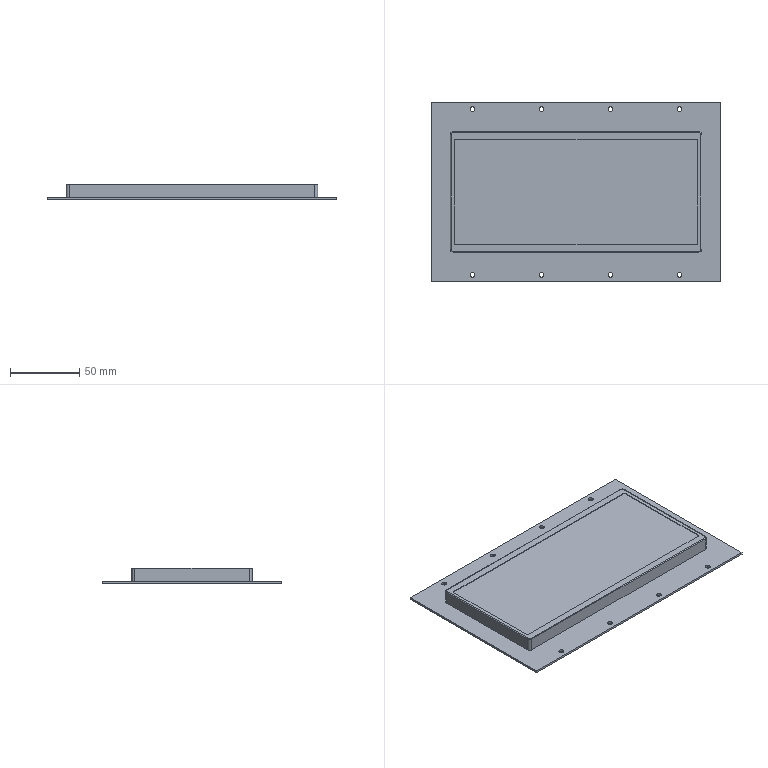Part | STEP file | 6151211W | 1 solid | 40 faces | box 210 x 130 x 11.5 mm | volume 192424 mm3 | cylinder 20 | plane 16 | torus 4 | commonest cylinder face diameters 3.5 x8 1 x4 2 x4 4 x4
STEP:
#1=CARTESIAN_POINT('',(-73.25,-60.,1.5));
#2=VERTEX_POINT('',#1);
#3=CARTESIAN_POINT('',(-75.,-60.,1.5));
#4=DIRECTION('',(0.,0.,1.));
#5=DIRECTION('',(1.,0.,0.));
#6=AXIS2_PLACEMENT_3D('',#3,#4,#5);
#7=CIRCLE('',#6,1.75);
#8=EDGE_CURVE('',#2,#2,#7,.T.);
#9=ORIENTED_EDGE('',*,*,#8,.F.);
#10=EDGE_LOOP('',(#9));
#11=FACE_BOUND('',#10,.T.);
#12=CARTESIAN_POINT('',(76.75,-60.,1.5));
#13=VERTEX_POINT('',#12);
#14=CARTESIAN_POINT('',(75.,-60.,1.5));
#15=DIRECTION('',(0.,0.,1.));
#16=DIRECTION('',(1.,0.,0.));
#17=AXIS2_PLACEMENT_3D('',#14,#15,#16);
#18=CIRCLE('',#17,1.75);
#19=EDGE_CURVE('',#13,#13,#18,.T.);
#20=ORIENTED_EDGE('',*,*,#19,.F.);
#21=EDGE_LOOP('',(#20));
#22=FACE_BOUND('',#21,.T.);
#23=CARTESIAN_POINT('',(26.75,60.,1.5));
#24=VERTEX_POINT('',#23);
#25=CARTESIAN_POINT('',(25.,60.,1.5));
#26=DIRECTION('',(0.,0.,1.));
#27=DIRECTION('',(1.,0.,0.));
#28=AXIS2_PLACEMENT_3D('',#25,#26,#27);
#29=CIRCLE('',#28,1.75);
#30=EDGE_CURVE('',#24,#24,#29,.T.);
#31=ORIENTED_EDGE('',*,*,#30,.F.);
#32=EDGE_LOOP('',(#31));
#33=FACE_BOUND('',#32,.T.);
#34=CARTESIAN_POINT('',(-23.25,60.,1.5));
#35=VERTEX_POINT('',#34);
#36=CARTESIAN_POINT('',(-25.,60.,1.5));
#37=DIRECTION('',(0.,0.,1.));
#38=DIRECTION('',(1.,0.,0.));
#39=AXIS2_PLACEMENT_3D('',#36,#37,#38);
#40=CIRCLE('',#39,1.75);
#41=EDGE_CURVE('',#35,#35,#40,.T.);
#42=ORIENTED_EDGE('',*,*,#41,.F.);
#43=EDGE_LOOP('',(#42));
#44=FACE_BOUND('',#43,.T.);
#45=CARTESIAN_POINT('',(-23.25,-60.,1.5));
#46=VERTEX_POINT('',#45);
#47=CARTESIAN_POINT('',(-25.,-60.,1.5));
#48=DIRECTION('',(0.,0.,1.));
#49=DIRECTION('',(1.,0.,0.));
#50=AXIS2_PLACEMENT_3D('',#47,#48,#49);
#51=CIRCLE('',#50,1.75);
#52=EDGE_CURVE('',#46,#46,#51,.T.);
#53=ORIENTED_EDGE('',*,*,#52,.F.);
#54=EDGE_LOOP('',(#53));
#55=FACE_BOUND('',#54,.T.);
#56=CARTESIAN_POINT('',(26.75,-60.,1.5));
#57=VERTEX_POINT('',#56);
#58=CARTESIAN_POINT('',(25.,-60.,1.5));
#59=DIRECTION('',(0.,0.,1.));
#60=DIRECTION('',(1.,0.,0.));
#61=AXIS2_PLACEMENT_3D('',#58,#59,#60);
#62=CIRCLE('',#61,1.75);
#63=EDGE_CURVE('',#57,#57,#62,.T.);
#64=ORIENTED_EDGE('',*,*,#63,.F.);
#65=EDGE_LOOP('',(#64));
#66=FACE_BOUND('',#65,.T.);
#67=CARTESIAN_POINT('',(76.75,60.,1.5));
#68=VERTEX_POINT('',#67);
#69=CARTESIAN_POINT('',(75.,60.,1.5));
#70=DIRECTION('',(0.,0.,1.));
#71=DIRECTION('',(1.,0.,0.));
#72=AXIS2_PLACEMENT_3D('',#69,#70,#71);
#73=CIRCLE('',#72,1.75);
#74=EDGE_CURVE('',#68,#68,#73,.T.);
#75=ORIENTED_EDGE('',*,*,#74,.F.);
#76=EDGE_LOOP('',(#75));
#77=FACE_BOUND('',#76,.T.);
#78=CARTESIAN_POINT('',(-73.25,60.,1.5));
#79=VERTEX_POINT('',#78);
#80=CARTESIAN_POINT('',(-75.,60.,1.5));
#81=DIRECTION('',(0.,0.,1.));
#82=DIRECTION('',(1.,0.,0.));
#83=AXIS2_PLACEMENT_3D('',#80,#81,#82);
#84=CIRCLE('',#83,1.75);
#85=EDGE_CURVE('',#79,#79,#84,.T.);
#86=ORIENTED_EDGE('',*,*,#85,.F.);
#87=EDGE_LOOP('',(#86));
#88=FACE_BOUND('',#87,.T.);
#89=CARTESIAN_POINT('',(-105.,65.,1.5));
#90=VERTEX_POINT('',#89);
#91=CARTESIAN_POINT('',(-105.,-65.,1.5));
#92=VERTEX_POINT('',#91);
#93=CARTESIAN_POINT('',(-105.,65.,1.5));
#94=DIRECTION('',(0.,-1.,0.));
#95=VECTOR('',#94,1000.);
#96=LINE('',#93,#95);
#97=EDGE_CURVE('',#90,#92,#96,.T.);
#98=ORIENTED_EDGE('',*,*,#97,.T.);
#99=CARTESIAN_POINT('',(105.,-65.,1.5));
#100=VERTEX_POINT('',#99);
#101=CARTESIAN_POINT('',(-105.,-65.,1.5));
#102=DIRECTION('',(1.,0.,0.));
#103=VECTOR('',#102,1000.);
#104=LINE('',#101,#103);
#105=EDGE_CURVE('',#92,#100,#104,.T.);
#106=ORIENTED_EDGE('',*,*,#105,.T.);
#107=CARTESIAN_POINT('',(105.,65.,1.5));
#108=VERTEX_POINT('',#107);
#109=CARTESIAN_POINT('',(105.,65.,1.5));
#110=DIRECTION('',(0.,1.,0.));
#111=VECTOR('',#110,1000.);
#112=LINE('',#109,#111);
#113=EDGE_CURVE('',#100,#108,#112,.T.);
#114=ORIENTED_EDGE('',*,*,#113,.T.);
#115=CARTESIAN_POINT('',(-105.,65.,1.5));
#116=DIRECTION('',(-1.,0.,0.));
#117=VECTOR('',#116,1000.);
#118=LINE('',#115,#117);
#119=EDGE_CURVE('',#108,#90,#118,.T.);
#120=ORIENTED_EDGE('',*,*,#119,.T.);
#121=EDGE_LOOP('',(#98,#106,#114,#120));
#122=FACE_OUTER_BOUND('',#121,.T.);
#123=CARTESIAN_POINT('',(89.,43.5,1.5));
#124=VERTEX_POINT('',#123);
#125=CARTESIAN_POINT('',(-89.,43.5,1.5));
#126=VERTEX_POINT('',#125);
#127=CARTESIAN_POINT('',(-89.,43.5,1.5));
#128=DIRECTION('',(-1.,0.,0.));
#129=VECTOR('',#128,1000.);
#130=LINE('',#127,#129);
#131=EDGE_CURVE('',#124,#126,#130,.T.);
#132=ORIENTED_EDGE('',*,*,#131,.F.);
#133=CARTESIAN_POINT('',(91.,41.5,1.5));
#134=VERTEX_POINT('',#133);
#135=CARTESIAN_POINT('',(89.,41.5,1.5));
#136=DIRECTION('',(0.,0.,1.));
#137=DIRECTION('',(1.,0.,0.));
#138=AXIS2_PLACEMENT_3D('',#135,#136,#137);
#139=CIRCLE('',#138,2.);
#140=EDGE_CURVE('',#134,#124,#139,.T.);
#141=ORIENTED_EDGE('',*,*,#140,.F.);
#142=CARTESIAN_POINT('',(91.,-41.5,1.5));
#143=VERTEX_POINT('',#142);
#144=CARTESIAN_POINT('',(91.,41.5,1.5));
#145=DIRECTION('',(0.,1.,0.));
#146=VECTOR('',#145,1000.);
#147=LINE('',#144,#146);
#148=EDGE_CURVE('',#143,#134,#147,.T.);
#149=ORIENTED_EDGE('',*,*,#148,.F.);
#150=CARTESIAN_POINT('',(89.,-43.5,1.5));
#151=VERTEX_POINT('',#150);
#152=CARTESIAN_POINT('',(89.,-41.5,1.5));
#153=DIRECTION('',(0.,0.,1.));
#154=DIRECTION('',(1.,0.,0.));
#155=AXIS2_PLACEMENT_3D('',#152,#153,#154);
#156=CIRCLE('',#155,2.);
#157=EDGE_CURVE('',#151,#143,#156,.T.);
#158=ORIENTED_EDGE('',*,*,#157,.F.);
#159=CARTESIAN_POINT('',(-89.,-43.5,1.5));
#160=VERTEX_POINT('',#159);
#161=CARTESIAN_POINT('',(-89.,-43.5,1.5));
#162=DIRECTION('',(1.,0.,0.));
#163=VECTOR('',#162,1000.);
#164=LINE('',#161,#163);
#165=EDGE_CURVE('',#160,#151,#164,.T.);
#166=ORIENTED_EDGE('',*,*,#165,.F.);
#167=CARTESIAN_POINT('',(-91.,-41.5,1.5));
#168=VERTEX_POINT('',#167);
#169=CARTESIAN_POINT('',(-89.,-41.5,1.5));
#170=DIRECTION('',(0.,0.,1.));
#171=DIRECTION('',(1.,0.,0.));
#172=AXIS2_PLACEMENT_3D('',#169,#170,#171);
#173=CIRCLE('',#172,2.);
#174=EDGE_CURVE('',#168,#160,#173,.T.);
#175=ORIENTED_EDGE('',*,*,#174,.F.);
#176=CARTESIAN_POINT('',(-91.,41.5,1.5));
#177=VERTEX_POINT('',#176);
#178=CARTESIAN_POINT('',(-91.,41.5,1.5));
#179=DIRECTION('',(0.,-1.,0.));
#180=VECTOR('',#179,1000.);
#181=LINE('',#178,#180);
#182=EDGE_CURVE('',#177,#168,#181,.T.);
#183=ORIENTED_EDGE('',*,*,#182,.F.);
#184=CARTESIAN_POINT('',(-89.,41.5,1.5));
#185=DIRECTION('',(0.,0.,1.));
#186=DIRECTION('',(1.,0.,0.));
#187=AXIS2_PLACEMENT_3D('',#184,#185,#186);
#188=CIRCLE('',#187,2.);
#189=EDGE_CURVE('',#126,#177,#188,.T.);
#190=ORIENTED_EDGE('',*,*,#189,.F.);
#191=EDGE_LOOP('',(#132,#141,#149,#158,#166,#175,#183,#190));
#192=FACE_BOUND('',#191,.T.);
#193=CARTESIAN_POINT('',(-105.,-65.,1.5));
#194=DIRECTION('',(0.,0.,1.));
#195=DIRECTION('',(1.,0.,0.));
#196=AXIS2_PLACEMENT_3D('',#193,#194,#195);
#197=PLANE('',#196);
#198=ADVANCED_FACE('',(#11,#22,#33,#44,#55,#66,#77,#88,#122,#192),#197,.T.);
#199=CARTESIAN_POINT('',(-105.,65.,0.));
#200=VERTEX_POINT('',#199);
#201=CARTESIAN_POINT('',(-105.,-65.,0.));
#202=VERTEX_POINT('',#201);
#203=CARTESIAN_POINT('',(-105.,65.,0.));
#204=DIRECTION('',(0.,-1.,0.));
#205=VECTOR('',#204,1000.);
#206=LINE('',#203,#205);
#207=EDGE_CURVE('',#200,#202,#206,.T.);
#208=ORIENTED_EDGE('',*,*,#207,.T.);
#209=CARTESIAN_POINT('',(-105.,-65.,1.5));
#210=DIRECTION('',(0.,0.,-1.));
#211=VECTOR('',#210,1000.);
#212=LINE('',#209,#211);
#213=EDGE_CURVE('',#92,#202,#212,.T.);
#214=ORIENTED_EDGE('',*,*,#213,.F.);
#215=ORIENTED_EDGE('',*,*,#97,.F.);
#216=CARTESIAN_POINT('',(-105.,65.,1.5));
#217=DIRECTION('',(0.,0.,-1.));
#218=VECTOR('',#217,1000.);
#219=LINE('',#216,#218);
#220=EDGE_CURVE('',#90,#200,#219,.T.);
#221=ORIENTED_EDGE('',*,*,#220,.T.);
#222=EDGE_LOOP('',(#208,#214,#215,#221));
#223=FACE_OUTER_BOUND('',#222,.T.);
#224=CARTESIAN_POINT('',(-105.,65.,1.5));
#225=DIRECTION('',(1.,0.,0.));
#226=DIRECTION('',(0.,1.,0.));
#227=AXIS2_PLACEMENT_3D('',#224,#225,#226);
#228=PLANE('',#227);
#229=ADVANCED_FACE('',(#223),#228,.F.);
#230=CARTESIAN_POINT('',(105.,-65.,0.));
#231=VERTEX_POINT('',#230);
#232=CARTESIAN_POINT('',(-105.,-65.,0.));
#233=DIRECTION('',(1.,0.,0.));
#234=VECTOR('',#233,1000.);
#235=LINE('',#232,#234);
#236=EDGE_CURVE('',#202,#231,#235,.T.);
#237=ORIENTED_EDGE('',*,*,#236,.T.);
#238=CARTESIAN_POINT('',(105.,-65.,1.5));
#239=DIRECTION('',(0.,0.,-1.));
#240=VECTOR('',#239,1000.);
#241=LINE('',#238,#240);
#242=EDGE_CURVE('',#100,#231,#241,.T.);
#243=ORIENTED_EDGE('',*,*,#242,.F.);
#244=ORIENTED_EDGE('',*,*,#105,.F.);
#245=ORIENTED_EDGE('',*,*,#213,.T.);
#246=EDGE_LOOP('',(#237,#243,#244,#245));
#247=FACE_OUTER_BOUND('',#246,.T.);
#248=CARTESIAN_POINT('',(-105.,-65.,1.5));
#249=DIRECTION('',(0.,1.,0.));
#250=DIRECTION('',(0.,0.,1.));
#251=AXIS2_PLACEMENT_3D('',#248,#249,#250);
#252=PLANE('',#251);
#253=ADVANCED_FACE('',(#247),#252,.F.);
#254=CARTESIAN_POINT('',(105.,65.,0.));
#255=VERTEX_POINT('',#254);
#256=CARTESIAN_POINT('',(105.,65.,0.));
#257=DIRECTION('',(0.,1.,0.));
#258=VECTOR('',#257,1000.);
#259=LINE('',#256,#258);
#260=EDGE_CURVE('',#231,#255,#259,.T.);
#261=ORIENTED_EDGE('',*,*,#260,.T.);
#262=CARTESIAN_POINT('',(105.,65.,1.5));
#263=DIRECTION('',(0.,0.,-1.));
#264=VECTOR('',#263,1000.);
#265=LINE('',#262,#264);
#266=EDGE_CURVE('',#108,#255,#265,.T.);
#267=ORIENTED_EDGE('',*,*,#266,.F.);
#268=ORIENTED_EDGE('',*,*,#113,.F.);
#269=ORIENTED_EDGE('',*,*,#242,.T.);
#270=EDGE_LOOP('',(#261,#267,#268,#269));
#271=FACE_OUTER_BOUND('',#270,.T.);
#272=CARTESIAN_POINT('',(105.,65.,1.5));
#273=DIRECTION('',(-1.,0.,0.));
#274=DIRECTION('',(0.,-1.,0.));
#275=AXIS2_PLACEMENT_3D('',#272,#273,#274);
#276=PLANE('',#275);
#277=ADVANCED_FACE('',(#271),#276,.F.);
#278=CARTESIAN_POINT('',(-105.,65.,0.));
#279=DIRECTION('',(-1.,0.,0.));
#280=VECTOR('',#279,1000.);
#281=LINE('',#278,#280);
#282=EDGE_CURVE('',#255,#200,#281,.T.);
#283=ORIENTED_EDGE('',*,*,#282,.T.);
#284=ORIENTED_EDGE('',*,*,#220,.F.);
#285=ORIENTED_EDGE('',*,*,#119,.F.);
#286=ORIENTED_EDGE('',*,*,#266,.T.);
#287=EDGE_LOOP('',(#283,#284,#285,#286));
#288=FACE_OUTER_BOUND('',#287,.T.);
#289=CARTESIAN_POINT('',(-105.,65.,1.5));
#290=DIRECTION('',(0.,-1.,0.));
#291=DIRECTION('',(0.,0.,-1.));
#292=AXIS2_PLACEMENT_3D('',#289,#290,#291);
#293=PLANE('',#292);
#294=ADVANCED_FACE('',(#288),#293,.F.);
#295=CARTESIAN_POINT('',(-73.25,-60.,0.));
#296=VERTEX_POINT('',#295);
#297=CARTESIAN_POINT('',(-75.,-60.,0.));
#298=DIRECTION('',(0.,0.,-1.));
#299=DIRECTION('',(1.,0.,0.));
#300=AXIS2_PLACEMENT_3D('',#297,#298,#299);
#301=CIRCLE('',#300,1.75);
#302=EDGE_CURVE('',#296,#296,#301,.T.);
#303=ORIENTED_EDGE('',*,*,#302,.F.);
#304=EDGE_LOOP('',(#303));
#305=FACE_BOUND('',#304,.T.);
#306=CARTESIAN_POINT('',(76.75,-60.,0.));
#307=VERTEX_POINT('',#306);
#308=CARTESIAN_POINT('',(75.,-60.,0.));
#309=DIRECTION('',(0.,0.,-1.));
#310=DIRECTION('',(1.,0.,0.));
#311=AXIS2_PLACEMENT_3D('',#308,#309,#310);
#312=CIRCLE('',#311,1.75);
#313=EDGE_CURVE('',#307,#307,#312,.T.);
#314=ORIENTED_EDGE('',*,*,#313,.F.);
#315=EDGE_LOOP('',(#314));
#316=FACE_BOUND('',#315,.T.);
#317=CARTESIAN_POINT('',(23.25,60.,0.));
#318=VERTEX_POINT('',#317);
#319=CARTESIAN_POINT('',(25.,60.,0.));
#320=DIRECTION('',(0.,0.,-1.));
#321=DIRECTION('',(-1.,0.,0.));
#322=AXIS2_PLACEMENT_3D('',#319,#320,#321);
#323=CIRCLE('',#322,1.75);
#324=EDGE_CURVE('',#318,#318,#323,.T.);
#325=ORIENTED_EDGE('',*,*,#324,.F.);
#326=EDGE_LOOP('',(#325));
#327=FACE_BOUND('',#326,.T.);
#328=CARTESIAN_POINT('',(-26.75,60.,0.));
#329=VERTEX_POINT('',#328);
#330=CARTESIAN_POINT('',(-25.,60.,0.));
#331=DIRECTION('',(0.,0.,-1.));
#332=DIRECTION('',(-1.,0.,0.));
#333=AXIS2_PLACEMENT_3D('',#330,#331,#332);
#334=CIRCLE('',#333,1.75);
#335=EDGE_CURVE('',#329,#329,#334,.T.);
#336=ORIENTED_EDGE('',*,*,#335,.F.);
#337=EDGE_LOOP('',(#336));
#338=FACE_BOUND('',#337,.T.);
#339=CARTESIAN_POINT('',(-23.25,-60.,0.));
#340=VERTEX_POINT('',#339);
#341=CARTESIAN_POINT('',(-25.,-60.,0.));
#342=DIRECTION('',(0.,0.,-1.));
#343=DIRECTION('',(1.,0.,0.));
#344=AXIS2_PLACEMENT_3D('',#341,#342,#343);
#345=CIRCLE('',#344,1.75);
#346=EDGE_CURVE('',#340,#340,#345,.T.);
#347=ORIENTED_EDGE('',*,*,#346,.F.);
#348=EDGE_LOOP('',(#347));
#349=FACE_BOUND('',#348,.T.);
#350=CARTESIAN_POINT('',(26.75,-60.,0.));
#351=VERTEX_POINT('',#350);
#352=CARTESIAN_POINT('',(25.,-60.,0.));
#353=DIRECTION('',(0.,0.,-1.));
#354=DIRECTION('',(1.,0.,0.));
#355=AXIS2_PLACEMENT_3D('',#352,#353,#354);
#356=CIRCLE('',#355,1.75);
#357=EDGE_CURVE('',#351,#351,#356,.T.);
#358=ORIENTED_EDGE('',*,*,#357,.F.);
#359=EDGE_LOOP('',(#358));
#360=FACE_BOUND('',#359,.T.);
#361=CARTESIAN_POINT('',(73.25,60.,0.));
#362=VERTEX_POINT('',#361);
#363=CARTESIAN_POINT('',(75.,60.,0.));
#364=DIRECTION('',(0.,0.,-1.));
#365=DIRECTION('',(-1.,0.,0.));
#366=AXIS2_PLACEMENT_3D('',#363,#364,#365);
#367=CIRCLE('',#366,1.75);
#368=EDGE_CURVE('',#362,#362,#367,.T.);
#369=ORIENTED_EDGE('',*,*,#368,.F.);
#370=EDGE_LOOP('',(#369));
#371=FACE_BOUND('',#370,.T.);
#372=CARTESIAN_POINT('',(-76.75,60.,0.));
#373=VERTEX_POINT('',#372);
#374=CARTESIAN_POINT('',(-75.,60.,0.));
#375=DIRECTION('',(0.,0.,-1.));
#376=DIRECTION('',(-1.,0.,0.));
#377=AXIS2_PLACEMENT_3D('',#374,#375,#376);
#378=CIRCLE('',#377,1.75);
#379=EDGE_CURVE('',#373,#373,#378,.T.);
#380=ORIENTED_EDGE('',*,*,#379,.F.);
#381=EDGE_LOOP('',(#380));
#382=FACE_BOUND('',#381,.T.);
#383=ORIENTED_EDGE('',*,*,#207,.F.);
#384=ORIENTED_EDGE('',*,*,#282,.F.);
#385=ORIENTED_EDGE('',*,*,#260,.F.);
#386=ORIENTED_EDGE('',*,*,#236,.F.);
#387=EDGE_LOOP('',(#383,#384,#385,#386));
#388=FACE_OUTER_BOUND('',#387,.T.);
#389=CARTESIAN_POINT('',(-105.,-65.,0.));
#390=DIRECTION('',(0.,0.,1.));
#391=DIRECTION('',(1.,0.,0.));
#392=AXIS2_PLACEMENT_3D('',#389,#390,#391);
#393=PLANE('',#392);
#394=ADVANCED_FACE('',(#305,#316,#327,#338,#349,#360,#371,#382,#388),#393,.F.);
#395=CARTESIAN_POINT('',(89.,43.5,11.));
#396=VERTEX_POINT('',#395);
#397=CARTESIAN_POINT('',(89.,43.5,11.5));
#398=DIRECTION('',(0.,0.,-1.));
#399=VECTOR('',#398,1000.);
#400=LINE('',#397,#399);
#401=EDGE_CURVE('',#396,#124,#400,.T.);
#402=ORIENTED_EDGE('',*,*,#401,.F.);
#403=CARTESIAN_POINT('',(91.,41.5,11.));
#404=VERTEX_POINT('',#403);
#405=CARTESIAN_POINT('',(89.,41.5,11.));
#406=DIRECTION('',(0.,0.,-1.));
#407=DIRECTION('',(1.,0.,0.));
#408=AXIS2_PLACEMENT_3D('',#405,#406,#407);
#409=CIRCLE('',#408,2.);
#410=EDGE_CURVE('',#396,#404,#409,.T.);
#411=ORIENTED_EDGE('',*,*,#410,.T.);
#412=CARTESIAN_POINT('',(91.,41.5,11.5));
#413=DIRECTION('',(0.,0.,-1.));
#414=VECTOR('',#413,1000.);
#415=LINE('',#412,#414);
#416=EDGE_CURVE('',#404,#134,#415,.T.);
#417=ORIENTED_EDGE('',*,*,#416,.T.);
#418=ORIENTED_EDGE('',*,*,#140,.T.);
#419=EDGE_LOOP('',(#402,#411,#417,#418));
#420=FACE_OUTER_BOUND('',#419,.T.);
#421=CARTESIAN_POINT('',(89.,41.5,11.5));
#422=DIRECTION('',(0.,0.,-1.));
#423=DIRECTION('',(-1.,0.,0.));
#424=AXIS2_PLACEMENT_3D('',#421,#422,#423);
#425=CYLINDRICAL_SURFACE('',#424,2.);
#426=ADVANCED_FACE('',(#420),#425,.T.);
#427=CARTESIAN_POINT('',(-89.,43.5,11.));
#428=VERTEX_POINT('',#427);
#429=CARTESIAN_POINT('',(-89.,43.5,11.5));
#430=DIRECTION('',(0.,0.,-1.));
#431=VECTOR('',#430,1000.);
#432=LINE('',#429,#431);
#433=EDGE_CURVE('',#428,#126,#432,.T.);
#434=ORIENTED_EDGE('',*,*,#433,.F.);
#435=CARTESIAN_POINT('',(89.,43.5,11.));
#436=DIRECTION('',(1.,0.,0.));
#437=VECTOR('',#436,1000.);
#438=LINE('',#435,#437);
#439=EDGE_CURVE('',#428,#396,#438,.T.);
#440=ORIENTED_EDGE('',*,*,#439,.T.);
#441=ORIENTED_EDGE('',*,*,#401,.T.);
#442=ORIENTED_EDGE('',*,*,#131,.T.);
#443=EDGE_LOOP('',(#434,#440,#441,#442));
#444=FACE_OUTER_BOUND('',#443,.T.);
#445=CARTESIAN_POINT('',(-89.,43.5,11.5));
#446=DIRECTION('',(0.,-1.,0.));
#447=DIRECTION('',(1.,0.,0.));
#448=AXIS2_PLACEMENT_3D('',#445,#446,#447);
#449=PLANE('',#448);
#450=ADVANCED_FACE('',(#444),#449,.F.);
#451=CARTESIAN_POINT('',(-91.,41.5,11.));
#452=VERTEX_POINT('',#451);
#453=CARTESIAN_POINT('',(-91.,41.5,11.5));
#454=DIRECTION('',(0.,0.,-1.));
#455=VECTOR('',#454,1000.);
#456=LINE('',#453,#455);
#457=EDGE_CURVE('',#452,#177,#456,.T.);
#458=ORIENTED_EDGE('',*,*,#457,.F.);
#459=CARTESIAN_POINT('',(-89.,41.5,11.));
#460=DIRECTION('',(0.,0.,-1.));
#461=DIRECTION('',(1.,0.,0.));
#462=AXIS2_PLACEMENT_3D('',#459,#460,#461);
#463=CIRCLE('',#462,2.);
#464=EDGE_CURVE('',#452,#428,#463,.T.);
#465=ORIENTED_EDGE('',*,*,#464,.T.);
#466=ORIENTED_EDGE('',*,*,#433,.T.);
#467=ORIENTED_EDGE('',*,*,#189,.T.);
#468=EDGE_LOOP('',(#458,#465,#466,#467));
#469=FACE_OUTER_BOUND('',#468,.T.);
#470=CARTESIAN_POINT('',(-89.,41.5,11.5));
#471=DIRECTION('',(0.,0.,-1.));
#472=DIRECTION('',(-1.,0.,0.));
#473=AXIS2_PLACEMENT_3D('',#470,#471,#472);
#474=CYLINDRICAL_SURFACE('',#473,2.);
#475=ADVANCED_FACE('',(#469),#474,.T.);
#476=CARTESIAN_POINT('',(-91.,-41.5,11.));
#477=VERTEX_POINT('',#476);
#478=CARTESIAN_POINT('',(-91.,-41.5,11.5));
#479=DIRECTION('',(0.,0.,-1.));
#480=VECTOR('',#479,1000.);
#481=LINE('',#478,#480);
#482=EDGE_CURVE('',#477,#168,#481,.T.);
#483=ORIENTED_EDGE('',*,*,#482,.F.);
#484=CARTESIAN_POINT('',(-91.,41.5,11.));
#485=DIRECTION('',(0.,1.,0.));
#486=VECTOR('',#485,1000.);
#487=LINE('',#484,#486);
#488=EDGE_CURVE('',#477,#452,#487,.T.);
#489=ORIENTED_EDGE('',*,*,#488,.T.);
#490=ORIENTED_EDGE('',*,*,#457,.T.);
#491=ORIENTED_EDGE('',*,*,#182,.T.);
#492=EDGE_LOOP('',(#483,#489,#490,#491));
#493=FACE_OUTER_BOUND('',#492,.T.);
#494=CARTESIAN_POINT('',(-91.,41.5,11.5));
#495=DIRECTION('',(1.,0.,0.));
#496=DIRECTION('',(0.,1.,0.));
#497=AXIS2_PLACEMENT_3D('',#494,#495,#496);
#498=PLANE('',#497);
#499=ADVANCED_FACE('',(#493),#498,.F.);
#500=CARTESIAN_POINT('',(-89.,-43.5,11.));
#501=VERTEX_POINT('',#500);
#502=CARTESIAN_POINT('',(-89.,-43.5,11.5));
#503=DIRECTION('',(0.,0.,-1.));
#504=VECTOR('',#503,1000.);
#505=LINE('',#502,#504);
#506=EDGE_CURVE('',#501,#160,#505,.T.);
#507=ORIENTED_EDGE('',*,*,#506,.F.);
#508=CARTESIAN_POINT('',(-89.,-41.5,11.));
#509=DIRECTION('',(0.,0.,-1.));
#510=DIRECTION('',(1.,0.,0.));
#511=AXIS2_PLACEMENT_3D('',#508,#509,#510);
#512=CIRCLE('',#511,2.);
#513=EDGE_CURVE('',#501,#477,#512,.T.);
#514=ORIENTED_EDGE('',*,*,#513,.T.);
#515=ORIENTED_EDGE('',*,*,#482,.T.);
#516=ORIENTED_EDGE('',*,*,#174,.T.);
#517=EDGE_LOOP('',(#507,#514,#515,#516));
#518=FACE_OUTER_BOUND('',#517,.T.);
#519=CARTESIAN_POINT('',(-89.,-41.5,11.5));
#520=DIRECTION('',(0.,0.,-1.));
#521=DIRECTION('',(-1.,0.,0.));
#522=AXIS2_PLACEMENT_3D('',#519,#520,#521);
#523=CYLINDRICAL_SURFACE('',#522,2.);
#524=ADVANCED_FACE('',(#518),#523,.T.);
#525=CARTESIAN_POINT('',(89.,-43.5,11.));
#526=VERTEX_POINT('',#525);
#527=CARTESIAN_POINT('',(89.,-43.5,11.5));
#528=DIRECTION('',(0.,0.,-1.));
#529=VECTOR('',#528,1000.);
#530=LINE('',#527,#529);
#531=EDGE_CURVE('',#526,#151,#530,.T.);
#532=ORIENTED_EDGE('',*,*,#531,.F.);
#533=CARTESIAN_POINT('',(-89.,-43.5,11.));
#534=DIRECTION('',(-1.,0.,0.));
#535=VECTOR('',#534,1000.);
#536=LINE('',#533,#535);
#537=EDGE_CURVE('',#526,#501,#536,.T.);
#538=ORIENTED_EDGE('',*,*,#537,.T.);
#539=ORIENTED_EDGE('',*,*,#506,.T.);
#540=ORIENTED_EDGE('',*,*,#165,.T.);
#541=EDGE_LOOP('',(#532,#538,#539,#540));
#542=FACE_OUTER_BOUND('',#541,.T.);
#543=CARTESIAN_POINT('',(-89.,-43.5,11.5));
#544=DIRECTION('',(0.,1.,0.));
#545=DIRECTION('',(-1.,0.,0.));
#546=AXIS2_PLACEMENT_3D('',#543,#544,#545);
#547=PLANE('',#546);
#548=ADVANCED_FACE('',(#542),#547,.F.);
#549=CARTESIAN_POINT('',(91.,-41.5,11.));
#550=VERTEX_POINT('',#549);
#551=CARTESIAN_POINT('',(91.,-41.5,11.5));
#552=DIRECTION('',(0.,0.,-1.));
#553=VECTOR('',#552,1000.);
#554=LINE('',#551,#553);
#555=EDGE_CURVE('',#550,#143,#554,.T.);
#556=ORIENTED_EDGE('',*,*,#555,.F.);
#557=CARTESIAN_POINT('',(89.,-41.5,11.));
#558=DIRECTION('',(0.,0.,-1.));
#559=DIRECTION('',(1.,0.,0.));
#560=AXIS2_PLACEMENT_3D('',#557,#558,#559);
#561=CIRCLE('',#560,2.);
#562=EDGE_CURVE('',#550,#526,#561,.T.);
#563=ORIENTED_EDGE('',*,*,#562,.T.);
#564=ORIENTED_EDGE('',*,*,#531,.T.);
#565=ORIENTED_EDGE('',*,*,#157,.T.);
#566=EDGE_LOOP('',(#556,#563,#564,#565));
#567=FACE_OUTER_BOUND('',#566,.T.);
#568=CARTESIAN_POINT('',(89.,-41.5,11.5));
#569=DIRECTION('',(0.,0.,-1.));
#570=DIRECTION('',(-1.,0.,0.));
#571=AXIS2_PLACEMENT_3D('',#568,#569,#570);
#572=CYLINDRICAL_SURFACE('',#571,2.);
#573=ADVANCED_FACE('',(#567),#572,.T.);
#574=ORIENTED_EDGE('',*,*,#416,.F.);
#575=CARTESIAN_POINT('',(91.,-41.5,11.));
#576=DIRECTION('',(0.,-1.,0.));
#577=VECTOR('',#576,1000.);
#578=LINE('',#575,#577);
#579=EDGE_CURVE('',#404,#550,#578,.T.);
#580=ORIENTED_EDGE('',*,*,#579,.T.);
#581=ORIENTED_EDGE('',*,*,#555,.T.);
#582=ORIENTED_EDGE('',*,*,#148,.T.);
#583=EDGE_LOOP('',(#574,#580,#581,#582));
#584=FACE_OUTER_BOUND('',#583,.T.);
#585=CARTESIAN_POINT('',(91.,41.5,11.5));
#586=DIRECTION('',(-1.,0.,0.));
#587=DIRECTION('',(0.,-1.,0.));
#588=AXIS2_PLACEMENT_3D('',#585,#586,#587);
#589=PLANE('',#588);
#590=ADVANCED_FACE('',(#584),#589,.F.);
#591=CARTESIAN_POINT('',(89.,43.,11.5));
#592=VERTEX_POINT('',#591);
#593=CARTESIAN_POINT('',(-89.,43.,11.5));
#594=VERTEX_POINT('',#593);
#595=CARTESIAN_POINT('',(-89.,43.,11.5));
#596=DIRECTION('',(-1.,0.,0.));
#597=VECTOR('',#596,1000.);
#598=LINE('',#595,#597);
#599=EDGE_CURVE('',#592,#594,#598,.T.);
#600=ORIENTED_EDGE('',*,*,#599,.T.);
#601=CARTESIAN_POINT('',(-90.5,41.5,11.5));
#602=VERTEX_POINT('',#601);
#603=CARTESIAN_POINT('',(-89.,41.5,11.5));
#604=DIRECTION('',(0.,0.,1.));
#605=DIRECTION('',(1.,0.,0.));
#606=AXIS2_PLACEMENT_3D('',#603,#604,#605);
#607=CIRCLE('',#606,1.5);
#608=EDGE_CURVE('',#594,#602,#607,.T.);
#609=ORIENTED_EDGE('',*,*,#608,.T.);
#610=CARTESIAN_POINT('',(-90.5,-41.5,11.5));
#611=VERTEX_POINT('',#610);
#612=CARTESIAN_POINT('',(-90.5,-41.5,11.5));
#613=DIRECTION('',(0.,-1.,0.));
#614=VECTOR('',#613,1000.);
#615=LINE('',#612,#614);
#616=EDGE_CURVE('',#602,#611,#615,.T.);
#617=ORIENTED_EDGE('',*,*,#616,.T.);
#618=CARTESIAN_POINT('',(-89.,-43.,11.5));
#619=VERTEX_POINT('',#618);
#620=CARTESIAN_POINT('',(-89.,-41.5,11.5));
#621=DIRECTION('',(0.,0.,1.));
#622=DIRECTION('',(1.,0.,0.));
#623=AXIS2_PLACEMENT_3D('',#620,#621,#622);
#624=CIRCLE('',#623,1.5);
#625=EDGE_CURVE('',#611,#619,#624,.T.);
#626=ORIENTED_EDGE('',*,*,#625,.T.);
#627=CARTESIAN_POINT('',(89.,-43.,11.5));
#628=VERTEX_POINT('',#627);
#629=CARTESIAN_POINT('',(89.,-43.,11.5));
#630=DIRECTION('',(1.,0.,0.));
#631=VECTOR('',#630,1000.);
#632=LINE('',#629,#631);
#633=EDGE_CURVE('',#619,#628,#632,.T.);
#634=ORIENTED_EDGE('',*,*,#633,.T.);
#635=CARTESIAN_POINT('',(90.5,-41.5,11.5));
#636=VERTEX_POINT('',#635);
#637=CARTESIAN_POINT('',(89.,-41.5,11.5));
#638=DIRECTION('',(0.,0.,1.));
#639=DIRECTION('',(1.,0.,0.));
#640=AXIS2_PLACEMENT_3D('',#637,#638,#639);
#641=CIRCLE('',#640,1.5);
#642=EDGE_CURVE('',#628,#636,#641,.T.);
#643=ORIENTED_EDGE('',*,*,#642,.T.);
#644=CARTESIAN_POINT('',(90.5,41.5,11.5));
#645=VERTEX_POINT('',#644);
#646=CARTESIAN_POINT('',(90.5,41.5,11.5));
#647=DIRECTION('',(0.,1.,0.));
#648=VECTOR('',#647,1000.);
#649=LINE('',#646,#648);
#650=EDGE_CURVE('',#636,#645,#649,.T.);
#651=ORIENTED_EDGE('',*,*,#650,.T.);
#652=CARTESIAN_POINT('',(89.,41.5,11.5));
#653=DIRECTION('',(0.,0.,1.));
#654=DIRECTION('',(1.,0.,0.));
#655=AXIS2_PLACEMENT_3D('',#652,#653,#654);
#656=CIRCLE('',#655,1.5);
#657=EDGE_CURVE('',#645,#592,#656,.T.);
#658=ORIENTED_EDGE('',*,*,#657,.T.);
#659=EDGE_LOOP('',(#600,#609,#617,#626,#634,#643,#651,#658));
#660=FACE_OUTER_BOUND('',#659,.T.);
#661=CARTESIAN_POINT('',(-87.,38.,11.5));
#662=VERTEX_POINT('',#661);
#663=CARTESIAN_POINT('',(-88.,37.,11.5));
#664=VERTEX_POINT('',#663);
#665=CARTESIAN_POINT('',(-87.,37.,11.5));
#666=DIRECTION('',(0.,0.,1.));
#667=DIRECTION('',(1.,0.,0.));
#668=AXIS2_PLACEMENT_3D('',#665,#666,#667);
#669=CIRCLE('',#668,1.);
#670=EDGE_CURVE('',#662,#664,#669,.T.);
#671=ORIENTED_EDGE('',*,*,#670,.F.);
#672=CARTESIAN_POINT('',(87.,38.,11.5));
#673=VERTEX_POINT('',#672);
#674=CARTESIAN_POINT('',(-87.,38.,11.5));
#675=DIRECTION('',(-1.,0.,0.));
#676=VECTOR('',#675,1000.);
#677=LINE('',#674,#676);
#678=EDGE_CURVE('',#673,#662,#677,.T.);
#679=ORIENTED_EDGE('',*,*,#678,.F.);
#680=CARTESIAN_POINT('',(88.,37.,11.5));
#681=VERTEX_POINT('',#680);
#682=CARTESIAN_POINT('',(87.,37.,11.5));
#683=DIRECTION('',(0.,0.,1.));
#684=DIRECTION('',(-1.,0.,0.));
#685=AXIS2_PLACEMENT_3D('',#682,#683,#684);
#686=CIRCLE('',#685,1.);
#687=EDGE_CURVE('',#681,#673,#686,.T.);
#688=ORIENTED_EDGE('',*,*,#687,.F.);
#689=CARTESIAN_POINT('',(88.,-37.,11.5));
#690=VERTEX_POINT('',#689);
#691=CARTESIAN_POINT('',(88.,37.,11.5));
#692=DIRECTION('',(0.,1.,0.));
#693=VECTOR('',#692,1000.);
#694=LINE('',#691,#693);
#695=EDGE_CURVE('',#690,#681,#694,.T.);
#696=ORIENTED_EDGE('',*,*,#695,.F.);
#697=CARTESIAN_POINT('',(87.,-38.,11.5));
#698=VERTEX_POINT('',#697);
#699=CARTESIAN_POINT('',(87.,-37.,11.5));
#700=DIRECTION('',(0.,0.,1.));
#701=DIRECTION('',(1.,0.,0.));
#702=AXIS2_PLACEMENT_3D('',#699,#700,#701);
#703=CIRCLE('',#702,1.);
#704=EDGE_CURVE('',#698,#690,#703,.T.);
#705=ORIENTED_EDGE('',*,*,#704,.F.);
#706=CARTESIAN_POINT('',(-87.,-38.,11.5));
#707=VERTEX_POINT('',#706);
#708=CARTESIAN_POINT('',(-87.,-38.,11.5));
#709=DIRECTION('',(1.,0.,0.));
#710=VECTOR('',#709,1000.);
#711=LINE('',#708,#710);
#712=EDGE_CURVE('',#707,#698,#711,.T.);
#713=ORIENTED_EDGE('',*,*,#712,.F.);
#714=CARTESIAN_POINT('',(-88.,-37.,11.5));
#715=VERTEX_POINT('',#714);
#716=CARTESIAN_POINT('',(-87.,-37.,11.5));
#717=DIRECTION('',(0.,0.,1.));
#718=DIRECTION('',(1.,0.,0.));
#719=AXIS2_PLACEMENT_3D('',#716,#717,#718);
#720=CIRCLE('',#719,1.);
#721=EDGE_CURVE('',#715,#707,#720,.T.);
#722=ORIENTED_EDGE('',*,*,#721,.F.);
#723=CARTESIAN_POINT('',(-88.,37.,11.5));
#724=DIRECTION('',(0.,-1.,0.));
#725=VECTOR('',#724,1000.);
#726=LINE('',#723,#725);
#727=EDGE_CURVE('',#664,#715,#726,.T.);
#728=ORIENTED_EDGE('',*,*,#727,.F.);
#729=EDGE_LOOP('',(#671,#679,#688,#696,#705,#713,#722,#728));
#730=FACE_BOUND('',#729,.T.);
#731=CARTESIAN_POINT('',(89.,41.5,11.5));
#732=DIRECTION('',(0.,0.,1.));
#733=DIRECTION('',(1.,0.,0.));
#734=AXIS2_PLACEMENT_3D('',#731,#732,#733);
#735=PLANE('',#734);
#736=ADVANCED_FACE('',(#660,#730),#735,.T.);
#737=ORIENTED_EDGE('',*,*,#670,.T.);
#738=CARTESIAN_POINT('',(-88.,37.,11.));
#739=VERTEX_POINT('',#738);
#740=CARTESIAN_POINT('',(-88.,37.,11.));
#741=DIRECTION('',(0.,0.,1.));
#742=VECTOR('',#741,1000.);
#743=LINE('',#740,#742);
#744=EDGE_CURVE('',#739,#664,#743,.T.);
#745=ORIENTED_EDGE('',*,*,#744,.F.);
#746=CARTESIAN_POINT('',(-87.,38.,11.));
#747=VERTEX_POINT('',#746);
#748=CARTESIAN_POINT('',(-87.,37.,11.));
#749=DIRECTION('',(0.,0.,1.));
#750=DIRECTION('',(1.,0.,0.));
#751=AXIS2_PLACEMENT_3D('',#748,#749,#750);
#752=CIRCLE('',#751,1.);
#753=EDGE_CURVE('',#747,#739,#752,.T.);
#754=ORIENTED_EDGE('',*,*,#753,.F.);
#755=CARTESIAN_POINT('',(-87.,38.,11.));
#756=DIRECTION('',(0.,0.,1.));
#757=VECTOR('',#756,1000.);
#758=LINE('',#755,#757);
#759=EDGE_CURVE('',#747,#662,#758,.T.);
#760=ORIENTED_EDGE('',*,*,#759,.T.);
#761=EDGE_LOOP('',(#737,#745,#754,#760));
#762=FACE_OUTER_BOUND('',#761,.T.);
#763=CARTESIAN_POINT('',(-87.,37.,11.));
#764=DIRECTION('',(0.,0.,1.));
#765=DIRECTION('',(1.,0.,0.));
#766=AXIS2_PLACEMENT_3D('',#763,#764,#765);
#767=CYLINDRICAL_SURFACE('',#766,1.);
#768=ADVANCED_FACE('',(#762),#767,.F.);
#769=ORIENTED_EDGE('',*,*,#678,.T.);
#770=ORIENTED_EDGE('',*,*,#759,.F.);
#771=CARTESIAN_POINT('',(87.,38.,11.));
#772=VERTEX_POINT('',#771);
#773=CARTESIAN_POINT('',(-87.,38.,11.));
#774=DIRECTION('',(-1.,0.,0.));
#775=VECTOR('',#774,1000.);
#776=LINE('',#773,#775);
#777=EDGE_CURVE('',#772,#747,#776,.T.);
#778=ORIENTED_EDGE('',*,*,#777,.F.);
#779=CARTESIAN_POINT('',(87.,38.,11.));
#780=DIRECTION('',(0.,0.,1.));
#781=VECTOR('',#780,1000.);
#782=LINE('',#779,#781);
#783=EDGE_CURVE('',#772,#673,#782,.T.);
#784=ORIENTED_EDGE('',*,*,#783,.T.);
#785=EDGE_LOOP('',(#769,#770,#778,#784));
#786=FACE_OUTER_BOUND('',#785,.T.);
#787=CARTESIAN_POINT('',(-87.,38.,11.));
#788=DIRECTION('',(0.,1.,0.));
#789=DIRECTION('',(0.,0.,1.));
#790=AXIS2_PLACEMENT_3D('',#787,#788,#789);
#791=PLANE('',#790);
#792=ADVANCED_FACE('',(#786),#791,.F.);
#793=ORIENTED_EDGE('',*,*,#687,.T.);
#794=ORIENTED_EDGE('',*,*,#783,.F.);
#795=CARTESIAN_POINT('',(88.,37.,11.));
#796=VERTEX_POINT('',#795);
#797=CARTESIAN_POINT('',(87.,37.,11.));
#798=DIRECTION('',(0.,0.,1.));
#799=DIRECTION('',(-1.,0.,0.));
#800=AXIS2_PLACEMENT_3D('',#797,#798,#799);
#801=CIRCLE('',#800,1.);
#802=EDGE_CURVE('',#796,#772,#801,.T.);
#803=ORIENTED_EDGE('',*,*,#802,.F.);
#804=CARTESIAN_POINT('',(88.,37.,11.));
#805=DIRECTION('',(0.,0.,1.));
#806=VECTOR('',#805,1000.);
#807=LINE('',#804,#806);
#808=EDGE_CURVE('',#796,#681,#807,.T.);
#809=ORIENTED_EDGE('',*,*,#808,.T.);
#810=EDGE_LOOP('',(#793,#794,#803,#809));
#811=FACE_OUTER_BOUND('',#810,.T.);
#812=CARTESIAN_POINT('',(87.,37.,11.));
#813=DIRECTION('',(0.,0.,1.));
#814=DIRECTION('',(1.,0.,0.));
#815=AXIS2_PLACEMENT_3D('',#812,#813,#814);
#816=CYLINDRICAL_SURFACE('',#815,1.);
#817=ADVANCED_FACE('',(#811),#816,.F.);
#818=ORIENTED_EDGE('',*,*,#695,.T.);
#819=ORIENTED_EDGE('',*,*,#808,.F.);
#820=CARTESIAN_POINT('',(88.,-37.,11.));
#821=VERTEX_POINT('',#820);
#822=CARTESIAN_POINT('',(88.,37.,11.));
#823=DIRECTION('',(0.,1.,0.));
#824=VECTOR('',#823,1000.);
#825=LINE('',#822,#824);
#826=EDGE_CURVE('',#821,#796,#825,.T.);
#827=ORIENTED_EDGE('',*,*,#826,.F.);
#828=CARTESIAN_POINT('',(88.,-37.,11.));
#829=DIRECTION('',(0.,0.,1.));
#830=VECTOR('',#829,1000.);
#831=LINE('',#828,#830);
#832=EDGE_CURVE('',#821,#690,#831,.T.);
#833=ORIENTED_EDGE('',*,*,#832,.T.);
#834=EDGE_LOOP('',(#818,#819,#827,#833));
#835=FACE_OUTER_BOUND('',#834,.T.);
#836=CARTESIAN_POINT('',(88.,37.,11.));
#837=DIRECTION('',(1.,0.,0.));
#838=DIRECTION('',(0.,1.,0.));
#839=AXIS2_PLACEMENT_3D('',#836,#837,#838);
#840=PLANE('',#839);
#841=ADVANCED_FACE('',(#835),#840,.F.);
#842=ORIENTED_EDGE('',*,*,#704,.T.);
#843=ORIENTED_EDGE('',*,*,#832,.F.);
#844=CARTESIAN_POINT('',(87.,-38.,11.));
#845=VERTEX_POINT('',#844);
#846=CARTESIAN_POINT('',(87.,-37.,11.));
#847=DIRECTION('',(0.,0.,1.));
#848=DIRECTION('',(1.,0.,0.));
#849=AXIS2_PLACEMENT_3D('',#846,#847,#848);
#850=CIRCLE('',#849,1.);
#851=EDGE_CURVE('',#845,#821,#850,.T.);
#852=ORIENTED_EDGE('',*,*,#851,.F.);
#853=CARTESIAN_POINT('',(87.,-38.,11.));
#854=DIRECTION('',(0.,0.,1.));
#855=VECTOR('',#854,1000.);
#856=LINE('',#853,#855);
#857=EDGE_CURVE('',#845,#698,#856,.T.);
#858=ORIENTED_EDGE('',*,*,#857,.T.);
#859=EDGE_LOOP('',(#842,#843,#852,#858));
#860=FACE_OUTER_BOUND('',#859,.T.);
#861=CARTESIAN_POINT('',(87.,-37.,11.));
#862=DIRECTION('',(0.,0.,1.));
#863=DIRECTION('',(1.,0.,0.));
#864=AXIS2_PLACEMENT_3D('',#861,#862,#863);
#865=CYLINDRICAL_SURFACE('',#864,1.);
#866=ADVANCED_FACE('',(#860),#865,.F.);
#867=ORIENTED_EDGE('',*,*,#712,.T.);
#868=ORIENTED_EDGE('',*,*,#857,.F.);
#869=CARTESIAN_POINT('',(-87.,-38.,11.));
#870=VERTEX_POINT('',#869);
#871=CARTESIAN_POINT('',(-87.,-38.,11.));
#872=DIRECTION('',(1.,0.,0.));
#873=VECTOR('',#872,1000.);
#874=LINE('',#871,#873);
#875=EDGE_CURVE('',#870,#845,#874,.T.);
#876=ORIENTED_EDGE('',*,*,#875,.F.);
#877=CARTESIAN_POINT('',(-87.,-38.,11.));
#878=DIRECTION('',(0.,0.,1.));
#879=VECTOR('',#878,1000.);
#880=LINE('',#877,#879);
#881=EDGE_CURVE('',#870,#707,#880,.T.);
#882=ORIENTED_EDGE('',*,*,#881,.T.);
#883=EDGE_LOOP('',(#867,#868,#876,#882));
#884=FACE_OUTER_BOUND('',#883,.T.);
#885=CARTESIAN_POINT('',(-87.,-38.,11.));
#886=DIRECTION('',(0.,-1.,0.));
#887=DIRECTION('',(1.,0.,0.));
#888=AXIS2_PLACEMENT_3D('',#885,#886,#887);
#889=PLANE('',#888);
#890=ADVANCED_FACE('',(#884),#889,.F.);
#891=ORIENTED_EDGE('',*,*,#721,.T.);
#892=ORIENTED_EDGE('',*,*,#881,.F.);
#893=CARTESIAN_POINT('',(-88.,-37.,11.));
#894=VERTEX_POINT('',#893);
#895=CARTESIAN_POINT('',(-87.,-37.,11.));
#896=DIRECTION('',(0.,0.,1.));
#897=DIRECTION('',(1.,0.,0.));
#898=AXIS2_PLACEMENT_3D('',#895,#896,#897);
#899=CIRCLE('',#898,1.);
#900=EDGE_CURVE('',#894,#870,#899,.T.);
#901=ORIENTED_EDGE('',*,*,#900,.F.);
#902=CARTESIAN_POINT('',(-88.,-37.,11.));
#903=DIRECTION('',(0.,0.,1.));
#904=VECTOR('',#903,1000.);
#905=LINE('',#902,#904);
#906=EDGE_CURVE('',#894,#715,#905,.T.);
#907=ORIENTED_EDGE('',*,*,#906,.T.);
#908=EDGE_LOOP('',(#891,#892,#901,#907));
#909=FACE_OUTER_BOUND('',#908,.T.);
#910=CARTESIAN_POINT('',(-87.,-37.,11.));
#911=DIRECTION('',(0.,0.,1.));
#912=DIRECTION('',(1.,0.,0.));
#913=AXIS2_PLACEMENT_3D('',#910,#911,#912);
#914=CYLINDRICAL_SURFACE('',#913,1.);
#915=ADVANCED_FACE('',(#909),#914,.F.);
#916=ORIENTED_EDGE('',*,*,#727,.T.);
#917=ORIENTED_EDGE('',*,*,#906,.F.);
#918=CARTESIAN_POINT('',(-88.,37.,11.));
#919=DIRECTION('',(0.,-1.,0.));
#920=VECTOR('',#919,1000.);
#921=LINE('',#918,#920);
#922=EDGE_CURVE('',#739,#894,#921,.T.);
#923=ORIENTED_EDGE('',*,*,#922,.F.);
#924=ORIENTED_EDGE('',*,*,#744,.T.);
#925=EDGE_LOOP('',(#916,#917,#923,#924));
#926=FACE_OUTER_BOUND('',#925,.T.);
#927=CARTESIAN_POINT('',(-88.,37.,11.));
#928=DIRECTION('',(-1.,0.,0.));
#929=DIRECTION('',(0.,0.,1.));
#930=AXIS2_PLACEMENT_3D('',#927,#928,#929);
#931=PLANE('',#930);
#932=ADVANCED_FACE('',(#926),#931,.F.);
#933=ORIENTED_EDGE('',*,*,#753,.T.);
#934=ORIENTED_EDGE('',*,*,#922,.T.);
#935=ORIENTED_EDGE('',*,*,#900,.T.);
#936=ORIENTED_EDGE('',*,*,#875,.T.);
#937=ORIENTED_EDGE('',*,*,#851,.T.);
#938=ORIENTED_EDGE('',*,*,#826,.T.);
#939=ORIENTED_EDGE('',*,*,#802,.T.);
#940=ORIENTED_EDGE('',*,*,#777,.T.);
#941=EDGE_LOOP('',(#933,#934,#935,#936,#937,#938,#939,#940));
#942=FACE_OUTER_BOUND('',#941,.T.);
#943=CARTESIAN_POINT('',(-87.,37.,11.));
#944=DIRECTION('',(0.,0.,1.));
#945=DIRECTION('',(1.,0.,0.));
#946=AXIS2_PLACEMENT_3D('',#943,#944,#945);
#947=PLANE('',#946);
#948=ADVANCED_FACE('',(#942),#947,.T.);
#949=ORIENTED_EDGE('',*,*,#85,.T.);
#950=EDGE_LOOP('',(#949));
#951=FACE_OUTER_BOUND('',#950,.T.);
#952=ORIENTED_EDGE('',*,*,#379,.T.);
#953=EDGE_LOOP('',(#952));
#954=FACE_OUTER_BOUND('',#953,.T.);
#955=CARTESIAN_POINT('',(-75.,60.,3.5));
#956=DIRECTION('',(0.,0.,-1.));
#957=DIRECTION('',(-1.,0.,0.));
#958=AXIS2_PLACEMENT_3D('',#955,#956,#957);
#959=CYLINDRICAL_SURFACE('',#958,1.75);
#960=ADVANCED_FACE('',(#951,#954),#959,.F.);
#961=ORIENTED_EDGE('',*,*,#74,.T.);
#962=EDGE_LOOP('',(#961));
#963=FACE_OUTER_BOUND('',#962,.T.);
#964=ORIENTED_EDGE('',*,*,#368,.T.);
#965=EDGE_LOOP('',(#964));
#966=FACE_OUTER_BOUND('',#965,.T.);
#967=CARTESIAN_POINT('',(75.,60.,3.5));
#968=DIRECTION('',(0.,0.,-1.));
#969=DIRECTION('',(-1.,0.,0.));
#970=AXIS2_PLACEMENT_3D('',#967,#968,#969);
#971=CYLINDRICAL_SURFACE('',#970,1.75);
#972=ADVANCED_FACE('',(#963,#966),#971,.F.);
#973=ORIENTED_EDGE('',*,*,#63,.T.);
#974=EDGE_LOOP('',(#973));
#975=FACE_OUTER_BOUND('',#974,.T.);
#976=ORIENTED_EDGE('',*,*,#357,.T.);
#977=EDGE_LOOP('',(#976));
#978=FACE_OUTER_BOUND('',#977,.T.);
#979=CARTESIAN_POINT('',(25.,-60.,3.5));
#980=DIRECTION('',(0.,0.,-1.));
#981=DIRECTION('',(-1.,0.,0.));
#982=AXIS2_PLACEMENT_3D('',#979,#980,#981);
#983=CYLINDRICAL_SURFACE('',#982,1.75);
#984=ADVANCED_FACE('',(#975,#978),#983,.F.);
#985=ORIENTED_EDGE('',*,*,#52,.T.);
#986=EDGE_LOOP('',(#985));
#987=FACE_OUTER_BOUND('',#986,.T.);
#988=ORIENTED_EDGE('',*,*,#346,.T.);
#989=EDGE_LOOP('',(#988));
#990=FACE_OUTER_BOUND('',#989,.T.);
#991=CARTESIAN_POINT('',(-25.,-60.,3.5));
#992=DIRECTION('',(0.,0.,-1.));
#993=DIRECTION('',(-1.,0.,0.));
#994=AXIS2_PLACEMENT_3D('',#991,#992,#993);
#995=CYLINDRICAL_SURFACE('',#994,1.75);
#996=ADVANCED_FACE('',(#987,#990),#995,.F.);
#997=ORIENTED_EDGE('',*,*,#41,.T.);
#998=EDGE_LOOP('',(#997));
#999=FACE_OUTER_BOUND('',#998,.T.);
#1000=ORIENTED_EDGE('',*,*,#335,.T.);
#1001=EDGE_LOOP('',(#1000));
#1002=FACE_OUTER_BOUND('',#1001,.T.);
#1003=CARTESIAN_POINT('',(-25.,60.,3.5));
#1004=DIRECTION('',(0.,0.,-1.));
#1005=DIRECTION('',(-1.,0.,0.));
#1006=AXIS2_PLACEMENT_3D('',#1003,#1004,#1005);
#1007=CYLINDRICAL_SURFACE('',#1006,1.75);
#1008=ADVANCED_FACE('',(#999,#1002),#1007,.F.);
#1009=ORIENTED_EDGE('',*,*,#30,.T.);
#1010=EDGE_LOOP('',(#1009));
#1011=FACE_OUTER_BOUND('',#1010,.T.);
#1012=ORIENTED_EDGE('',*,*,#324,.T.);
#1013=EDGE_LOOP('',(#1012));
#1014=FACE_OUTER_BOUND('',#1013,.T.);
#1015=CARTESIAN_POINT('',(25.,60.,3.5));
#1016=DIRECTION('',(0.,0.,-1.));
#1017=DIRECTION('',(-1.,0.,0.));
#1018=AXIS2_PLACEMENT_3D('',#1015,#1016,#1017);
#1019=CYLINDRICAL_SURFACE('',#1018,1.75);
#1020=ADVANCED_FACE('',(#1011,#1014),#1019,.F.);
#1021=ORIENTED_EDGE('',*,*,#19,.T.);
#1022=EDGE_LOOP('',(#1021));
#1023=FACE_OUTER_BOUND('',#1022,.T.);
#1024=ORIENTED_EDGE('',*,*,#313,.T.);
#1025=EDGE_LOOP('',(#1024));
#1026=FACE_OUTER_BOUND('',#1025,.T.);
#1027=CARTESIAN_POINT('',(75.,-60.,3.5));
#1028=DIRECTION('',(0.,0.,-1.));
#1029=DIRECTION('',(-1.,0.,0.));
#1030=AXIS2_PLACEMENT_3D('',#1027,#1028,#1029);
#1031=CYLINDRICAL_SURFACE('',#1030,1.75);
#1032=ADVANCED_FACE('',(#1023,#1026),#1031,.F.);
#1033=ORIENTED_EDGE('',*,*,#8,.T.);
#1034=EDGE_LOOP('',(#1033));
#1035=FACE_OUTER_BOUND('',#1034,.T.);
#1036=ORIENTED_EDGE('',*,*,#302,.T.);
#1037=EDGE_LOOP('',(#1036));
#1038=FACE_OUTER_BOUND('',#1037,.T.);
#1039=CARTESIAN_POINT('',(-75.,-60.,3.5));
#1040=DIRECTION('',(0.,0.,-1.));
#1041=DIRECTION('',(-1.,0.,0.));
#1042=AXIS2_PLACEMENT_3D('',#1039,#1040,#1041);
#1043=CYLINDRICAL_SURFACE('',#1042,1.75);
#1044=ADVANCED_FACE('',(#1035,#1038),#1043,.F.);
#1045=CARTESIAN_POINT('',(89.,-43.,11.));
#1046=DIRECTION('',(-1.,0.,0.));
#1047=DIRECTION('',(0.,0.,1.));
#1048=AXIS2_PLACEMENT_3D('',#1045,#1046,#1047);
#1049=CIRCLE('',#1048,0.5);
#1050=EDGE_CURVE('',#526,#628,#1049,.T.);
#1051=ORIENTED_EDGE('',*,*,#1050,.F.);
#1052=ORIENTED_EDGE('',*,*,#562,.F.);
#1053=CARTESIAN_POINT('',(90.5,-41.5,11.));
#1054=DIRECTION('',(0.,1.,0.));
#1055=DIRECTION('',(0.,0.,1.));
#1056=AXIS2_PLACEMENT_3D('',#1053,#1054,#1055);
#1057=CIRCLE('',#1056,0.5);
#1058=EDGE_CURVE('',#636,#550,#1057,.T.);
#1059=ORIENTED_EDGE('',*,*,#1058,.F.);
#1060=ORIENTED_EDGE('',*,*,#642,.F.);
#1061=EDGE_LOOP('',(#1051,#1052,#1059,#1060));
#1062=FACE_OUTER_BOUND('',#1061,.T.);
#1063=CARTESIAN_POINT('',(89.,-41.5,11.));
#1064=DIRECTION('',(0.,0.,1.));
#1065=DIRECTION('',(1.,0.,0.));
#1066=AXIS2_PLACEMENT_3D('',#1063,#1064,#1065);
#1067=TOROIDAL_SURFACE('',#1066,1.5,0.5);
#1068=ADVANCED_FACE('',(#1062),#1067,.T.);
#1069=ORIENTED_EDGE('',*,*,#1058,.T.);
#1070=ORIENTED_EDGE('',*,*,#579,.F.);
#1071=CARTESIAN_POINT('',(90.5,41.5,11.));
#1072=DIRECTION('',(0.,1.,0.));
#1073=DIRECTION('',(0.,0.,1.));
#1074=AXIS2_PLACEMENT_3D('',#1071,#1072,#1073);
#1075=CIRCLE('',#1074,0.5);
#1076=EDGE_CURVE('',#645,#404,#1075,.T.);
#1077=ORIENTED_EDGE('',*,*,#1076,.F.);
#1078=ORIENTED_EDGE('',*,*,#650,.F.);
#1079=EDGE_LOOP('',(#1069,#1070,#1077,#1078));
#1080=FACE_OUTER_BOUND('',#1079,.T.);
#1081=CARTESIAN_POINT('',(90.5,41.5,11.));
#1082=DIRECTION('',(0.,-1.,0.));
#1083=DIRECTION('',(1.,0.,0.));
#1084=AXIS2_PLACEMENT_3D('',#1081,#1082,#1083);
#1085=CYLINDRICAL_SURFACE('',#1084,0.5);
#1086=ADVANCED_FACE('',(#1080),#1085,.T.);
#1087=ORIENTED_EDGE('',*,*,#1050,.T.);
#1088=ORIENTED_EDGE('',*,*,#633,.F.);
#1089=CARTESIAN_POINT('',(-89.,-43.,11.));
#1090=DIRECTION('',(-1.,0.,0.));
#1091=DIRECTION('',(0.,0.,1.));
#1092=AXIS2_PLACEMENT_3D('',#1089,#1090,#1091);
#1093=CIRCLE('',#1092,0.5);
#1094=EDGE_CURVE('',#501,#619,#1093,.T.);
#1095=ORIENTED_EDGE('',*,*,#1094,.F.);
#1096=ORIENTED_EDGE('',*,*,#537,.F.);
#1097=EDGE_LOOP('',(#1087,#1088,#1095,#1096));
#1098=FACE_OUTER_BOUND('',#1097,.T.);
#1099=CARTESIAN_POINT('',(89.,-43.,11.));
#1100=DIRECTION('',(-1.,0.,0.));
#1101=DIRECTION('',(0.,-1.,0.));
#1102=AXIS2_PLACEMENT_3D('',#1099,#1100,#1101);
#1103=CYLINDRICAL_SURFACE('',#1102,0.5);
#1104=ADVANCED_FACE('',(#1098),#1103,.T.);
#1105=ORIENTED_EDGE('',*,*,#1076,.T.);
#1106=ORIENTED_EDGE('',*,*,#410,.F.);
#1107=CARTESIAN_POINT('',(89.,43.,11.));
#1108=DIRECTION('',(-1.,0.,0.));
#1109=DIRECTION('',(0.,0.,1.));
#1110=AXIS2_PLACEMENT_3D('',#1107,#1108,#1109);
#1111=CIRCLE('',#1110,0.5);
#1112=EDGE_CURVE('',#592,#396,#1111,.T.);
#1113=ORIENTED_EDGE('',*,*,#1112,.F.);
#1114=ORIENTED_EDGE('',*,*,#657,.F.);
#1115=EDGE_LOOP('',(#1105,#1106,#1113,#1114));
#1116=FACE_OUTER_BOUND('',#1115,.T.);
#1117=CARTESIAN_POINT('',(89.,41.5,11.));
#1118=DIRECTION('',(0.,0.,1.));
#1119=DIRECTION('',(1.,0.,0.));
#1120=AXIS2_PLACEMENT_3D('',#1117,#1118,#1119);
#1121=TOROIDAL_SURFACE('',#1120,1.5,0.5);
#1122=ADVANCED_FACE('',(#1116),#1121,.T.);
#1123=ORIENTED_EDGE('',*,*,#1094,.T.);
#1124=ORIENTED_EDGE('',*,*,#625,.F.);
#1125=CARTESIAN_POINT('',(-90.5,-41.5,11.));
#1126=DIRECTION('',(0.,1.,0.));
#1127=DIRECTION('',(0.,0.,1.));
#1128=AXIS2_PLACEMENT_3D('',#1125,#1126,#1127);
#1129=CIRCLE('',#1128,0.5);
#1130=EDGE_CURVE('',#477,#611,#1129,.T.);
#1131=ORIENTED_EDGE('',*,*,#1130,.F.);
#1132=ORIENTED_EDGE('',*,*,#513,.F.);
#1133=EDGE_LOOP('',(#1123,#1124,#1131,#1132));
#1134=FACE_OUTER_BOUND('',#1133,.T.);
#1135=CARTESIAN_POINT('',(-89.,-41.5,11.));
#1136=DIRECTION('',(0.,0.,1.));
#1137=DIRECTION('',(1.,0.,0.));
#1138=AXIS2_PLACEMENT_3D('',#1135,#1136,#1137);
#1139=TOROIDAL_SURFACE('',#1138,1.5,0.5);
#1140=ADVANCED_FACE('',(#1134),#1139,.T.);
#1141=ORIENTED_EDGE('',*,*,#1112,.T.);
#1142=ORIENTED_EDGE('',*,*,#439,.F.);
#1143=CARTESIAN_POINT('',(-89.,43.,11.));
#1144=DIRECTION('',(-1.,0.,0.));
#1145=DIRECTION('',(0.,0.,1.));
#1146=AXIS2_PLACEMENT_3D('',#1143,#1144,#1145);
#1147=CIRCLE('',#1146,0.5);
#1148=EDGE_CURVE('',#594,#428,#1147,.T.);
#1149=ORIENTED_EDGE('',*,*,#1148,.F.);
#1150=ORIENTED_EDGE('',*,*,#599,.F.);
#1151=EDGE_LOOP('',(#1141,#1142,#1149,#1150));
#1152=FACE_OUTER_BOUND('',#1151,.T.);
#1153=CARTESIAN_POINT('',(89.,43.,11.));
#1154=DIRECTION('',(1.,0.,0.));
#1155=DIRECTION('',(0.,1.,0.));
#1156=AXIS2_PLACEMENT_3D('',#1153,#1154,#1155);
#1157=CYLINDRICAL_SURFACE('',#1156,0.5);
#1158=ADVANCED_FACE('',(#1152),#1157,.T.);
#1159=ORIENTED_EDGE('',*,*,#1130,.T.);
#1160=ORIENTED_EDGE('',*,*,#616,.F.);
#1161=CARTESIAN_POINT('',(-90.5,41.5,11.));
#1162=DIRECTION('',(0.,1.,0.));
#1163=DIRECTION('',(0.,0.,1.));
#1164=AXIS2_PLACEMENT_3D('',#1161,#1162,#1163);
#1165=CIRCLE('',#1164,0.5);
#1166=EDGE_CURVE('',#452,#602,#1165,.T.);
#1167=ORIENTED_EDGE('',*,*,#1166,.F.);
#1168=ORIENTED_EDGE('',*,*,#488,.F.);
#1169=EDGE_LOOP('',(#1159,#1160,#1167,#1168));
#1170=FACE_OUTER_BOUND('',#1169,.T.);
#1171=CARTESIAN_POINT('',(-90.5,41.5,11.));
#1172=DIRECTION('',(0.,1.,0.));
#1173=DIRECTION('',(-1.,0.,0.));
#1174=AXIS2_PLACEMENT_3D('',#1171,#1172,#1173);
#1175=CYLINDRICAL_SURFACE('',#1174,0.5);
#1176=ADVANCED_FACE('',(#1170),#1175,.T.);
#1177=ORIENTED_EDGE('',*,*,#1148,.T.);
#1178=ORIENTED_EDGE('',*,*,#464,.F.);
#1179=ORIENTED_EDGE('',*,*,#1166,.T.);
#1180=ORIENTED_EDGE('',*,*,#608,.F.);
#1181=EDGE_LOOP('',(#1177,#1178,#1179,#1180));
#1182=FACE_OUTER_BOUND('',#1181,.T.);
#1183=CARTESIAN_POINT('',(-89.,41.5,11.));
#1184=DIRECTION('',(0.,0.,1.));
#1185=DIRECTION('',(1.,0.,0.));
#1186=AXIS2_PLACEMENT_3D('',#1183,#1184,#1185);
#1187=TOROIDAL_SURFACE('',#1186,1.5,0.5);
#1188=ADVANCED_FACE('',(#1182),#1187,.T.);
#1189=CLOSED_SHELL('',(#198,#229,#253,#277,#294,#394,#426,#450,#475,#499,#524,#548,#573,#590,#736,#768,#792,#817,#841,#866,#890,#915,#932,#948,#960,#972,#984,#996,#1008,#1020,#1032,#1044,#1068,#1086,#1104,#1122,#1140,#1158,#1176,#1188));
#1190=MANIFOLD_SOLID_BREP('',#1189);
#1191=CARTESIAN_POINT('',(0.,0.,0.));
#1192=DIRECTION('',(0.,0.,1.));
#1193=DIRECTION('',(1.,0.,0.));
#1194=AXIS2_PLACEMENT_3D('',#1191,#1192,#1193);
#1195=(LENGTH_UNIT()NAMED_UNIT(*)SI_UNIT(.MILLI.,.METRE.));
#1196=UNCERTAINTY_MEASURE_WITH_UNIT(LENGTH_MEASURE(0.00001),#1195,'','');
#1197=(NAMED_UNIT(*)PLANE_ANGLE_UNIT()SI_UNIT($,.RADIAN.));
#1198=(NAMED_UNIT(*)SI_UNIT($,.STERADIAN.)SOLID_ANGLE_UNIT());
#1199=(GEOMETRIC_REPRESENTATION_CONTEXT(3)GLOBAL_UNCERTAINTY_ASSIGNED_CONTEXT((#1196))GLOBAL_UNIT_ASSIGNED_CONTEXT((#1195,#1197,#1198))REPRESENTATION_CONTEXT('',''));
#1200=ADVANCED_BREP_SHAPE_REPRESENTATION('',(#1190,#1194),#1199);